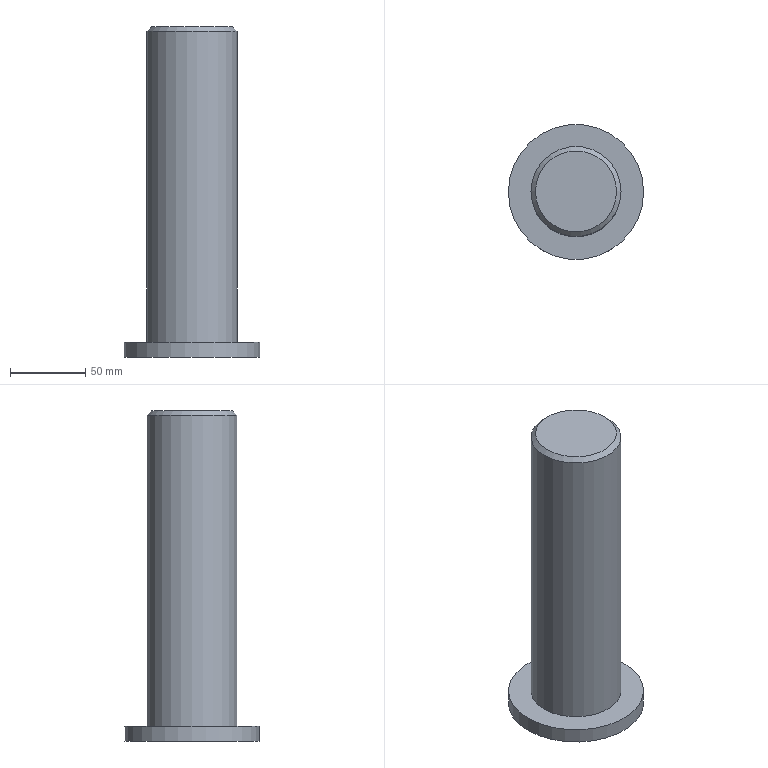Part | NX | features 推移杆连接头销柱 2 | 1 solid | 6 faces | box 90 x 90 x 220 mm | volume 656558 mm3 | plane 3 | cylinder 2 | cone 1 | commonest cylinder face diameters 60 x1 90 x1
STEP:
#1=CARTESIAN_POINT('',(30.,0.,207.));
#2=VERTEX_POINT('',#1);
#3=CARTESIAN_POINT('',(0.,0.,207.));
#4=DIRECTION('',(0.,0.,1.));
#5=DIRECTION('',(1.,0.,0.));
#6=AXIS2_PLACEMENT_3D('',#3,#4,#5);
#7=CIRCLE('',#6,30.);
#8=EDGE_CURVE('',#2,#2,#7,.F.);
#9=ORIENTED_EDGE('',*,*,#8,.T.);
#10=EDGE_LOOP('',(#9));
#11=FACE_BOUND('',#10,.T.);
#12=CARTESIAN_POINT('',(-30.,0.,0.));
#13=VERTEX_POINT('',#12);
#14=CARTESIAN_POINT('',(0.,0.,0.));
#15=DIRECTION('',(0.,0.,-1.));
#16=DIRECTION('',(-1.,0.,0.));
#17=AXIS2_PLACEMENT_3D('',#14,#15,#16);
#18=CIRCLE('',#17,30.);
#19=EDGE_CURVE('',#13,#13,#18,.T.);
#20=ORIENTED_EDGE('',*,*,#19,.F.);
#21=EDGE_LOOP('',(#20));
#22=FACE_BOUND('',#21,.T.);
#23=CARTESIAN_POINT('',(0.,0.,210.));
#24=DIRECTION('',(0.,0.,-1.));
#25=DIRECTION('',(-1.,0.,0.));
#26=AXIS2_PLACEMENT_3D('',#23,#24,#25);
#27=CYLINDRICAL_SURFACE('',#26,30.);
#28=ADVANCED_FACE('',(#11,#22),#27,.T.);
#29=CARTESIAN_POINT('',(27.,0.,210.));
#30=VERTEX_POINT('',#29);
#31=CARTESIAN_POINT('',(0.,0.,210.));
#32=DIRECTION('',(0.,0.,1.));
#33=DIRECTION('',(1.,0.,0.));
#34=AXIS2_PLACEMENT_3D('',#31,#32,#33);
#35=CIRCLE('',#34,27.);
#36=EDGE_CURVE('',#30,#30,#35,.T.);
#37=ORIENTED_EDGE('',*,*,#36,.T.);
#38=EDGE_LOOP('',(#37));
#39=FACE_BOUND('',#38,.T.);
#40=CARTESIAN_POINT('',(0.,0.,210.));
#41=DIRECTION('',(0.,0.,1.));
#42=DIRECTION('',(1.,0.,0.));
#43=AXIS2_PLACEMENT_3D('',#40,#41,#42);
#44=PLANE('',#43);
#45=ADVANCED_FACE('',(#39),#44,.T.);
#46=CARTESIAN_POINT('',(-45.,0.,0.));
#47=VERTEX_POINT('',#46);
#48=CARTESIAN_POINT('',(0.,0.,0.));
#49=DIRECTION('',(0.,0.,-1.));
#50=DIRECTION('',(-1.,0.,0.));
#51=AXIS2_PLACEMENT_3D('',#48,#49,#50);
#52=CIRCLE('',#51,45.);
#53=EDGE_CURVE('',#47,#47,#52,.T.);
#54=ORIENTED_EDGE('',*,*,#53,.F.);
#55=EDGE_LOOP('',(#54));
#56=FACE_BOUND('',#55,.T.);
#57=ORIENTED_EDGE('',*,*,#19,.T.);
#58=EDGE_LOOP('',(#57));
#59=FACE_BOUND('',#58,.T.);
#60=CARTESIAN_POINT('',(0.,0.,0.));
#61=DIRECTION('',(0.,0.,-1.));
#62=DIRECTION('',(-1.,0.,0.));
#63=AXIS2_PLACEMENT_3D('',#60,#61,#62);
#64=PLANE('',#63);
#65=ADVANCED_FACE('',(#56,#59),#64,.F.);
#66=CARTESIAN_POINT('',(-45.,0.,-10.));
#67=VERTEX_POINT('',#66);
#68=CARTESIAN_POINT('',(0.,0.,-10.));
#69=DIRECTION('',(0.,0.,-1.));
#70=DIRECTION('',(-1.,0.,0.));
#71=AXIS2_PLACEMENT_3D('',#68,#69,#70);
#72=CIRCLE('',#71,45.);
#73=EDGE_CURVE('',#67,#67,#72,.T.);
#74=ORIENTED_EDGE('',*,*,#73,.F.);
#75=EDGE_LOOP('',(#74));
#76=FACE_BOUND('',#75,.T.);
#77=ORIENTED_EDGE('',*,*,#53,.T.);
#78=EDGE_LOOP('',(#77));
#79=FACE_BOUND('',#78,.T.);
#80=CARTESIAN_POINT('',(0.,0.,-10.));
#81=DIRECTION('',(0.,0.,1.));
#82=DIRECTION('',(1.,0.,0.));
#83=AXIS2_PLACEMENT_3D('',#80,#81,#82);
#84=CYLINDRICAL_SURFACE('',#83,45.);
#85=ADVANCED_FACE('',(#76,#79),#84,.T.);
#86=ORIENTED_EDGE('',*,*,#73,.T.);
#87=EDGE_LOOP('',(#86));
#88=FACE_BOUND('',#87,.T.);
#89=CARTESIAN_POINT('',(0.,0.,-10.));
#90=DIRECTION('',(0.,0.,-1.));
#91=DIRECTION('',(-1.,0.,0.));
#92=AXIS2_PLACEMENT_3D('',#89,#90,#91);
#93=PLANE('',#92);
#94=ADVANCED_FACE('',(#88),#93,.T.);
#95=ORIENTED_EDGE('',*,*,#8,.F.);
#96=EDGE_LOOP('',(#95));
#97=FACE_BOUND('',#96,.T.);
#98=ORIENTED_EDGE('',*,*,#36,.F.);
#99=EDGE_LOOP('',(#98));
#100=FACE_BOUND('',#99,.T.);
#101=CARTESIAN_POINT('',(0.,0.,210.));
#102=DIRECTION('',(0.,0.,-1.));
#103=DIRECTION('',(-1.,0.,0.));
#104=AXIS2_PLACEMENT_3D('',#101,#102,#103);
#105=CONICAL_SURFACE('',#104,27.,0.7854);
#106=ADVANCED_FACE('',(#97,#100),#105,.T.);
#107=CLOSED_SHELL('',(#28,#45,#65,#85,#94,#106));
#108=MANIFOLD_SOLID_BREP('',#107);
#109=(LENGTH_UNIT()NAMED_UNIT(*)SI_UNIT(.MILLI.,.METRE.));
#110=UNCERTAINTY_MEASURE_WITH_UNIT(LENGTH_MEASURE(0.00001),#109,'','');
#111=(NAMED_UNIT(*)PLANE_ANGLE_UNIT()SI_UNIT($,.RADIAN.));
#112=(NAMED_UNIT(*)SI_UNIT($,.STERADIAN.)SOLID_ANGLE_UNIT());
#113=(GEOMETRIC_REPRESENTATION_CONTEXT(3)GLOBAL_UNCERTAINTY_ASSIGNED_CONTEXT((#110))GLOBAL_UNIT_ASSIGNED_CONTEXT((#109,#111,#112))REPRESENTATION_CONTEXT('',''));
#114=ADVANCED_BREP_SHAPE_REPRESENTATION('',(#108),#113);